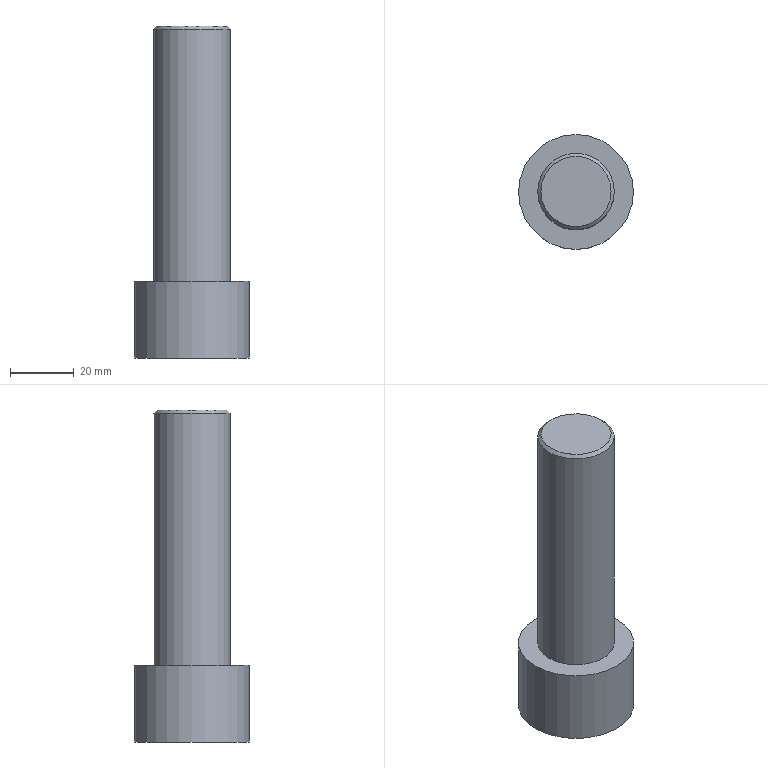Part | NX | features solid 2 | 1 solid | 16 faces | box 36 x 36 x 104 mm | volume 57183 mm3 | plane 11 | cylinder 4 | cone 1 | commonest cylinder face diameters 21.98 x1 22 x1 24 x1 36 x1
STEP:
#1=CARTESIAN_POINT('',(1313.5,-386.31,231.));
#2=VERTEX_POINT('',#1);
#3=CARTESIAN_POINT('',(1325.5,-386.31,231.));
#4=DIRECTION('',(0.,0.,-1.));
#5=DIRECTION('',(-1.,0.,0.));
#6=AXIS2_PLACEMENT_3D('',#3,#4,#5);
#7=CIRCLE('',#6,12.);
#8=EDGE_CURVE('',#2,#2,#7,.T.);
#9=ORIENTED_EDGE('',*,*,#8,.T.);
#10=EDGE_LOOP('',(#9));
#11=FACE_BOUND('',#10,.T.);
#12=CARTESIAN_POINT('',(1313.5,-386.31,152.));
#13=VERTEX_POINT('',#12);
#14=CARTESIAN_POINT('',(1325.5,-386.31,152.));
#15=DIRECTION('',(0.,0.,-1.));
#16=DIRECTION('',(-1.,0.,0.));
#17=AXIS2_PLACEMENT_3D('',#14,#15,#16);
#18=CIRCLE('',#17,12.);
#19=EDGE_CURVE('',#13,#13,#18,.F.);
#20=ORIENTED_EDGE('',*,*,#19,.T.);
#21=EDGE_LOOP('',(#20));
#22=FACE_BOUND('',#21,.T.);
#23=CARTESIAN_POINT('',(1325.5,-386.31,207.));
#24=DIRECTION('',(0.,0.,1.));
#25=DIRECTION('',(-1.,0.,0.));
#26=AXIS2_PLACEMENT_3D('',#23,#24,#25);
#27=CYLINDRICAL_SURFACE('',#26,12.);
#28=ADVANCED_FACE('',(#11,#22),#27,.T.);
#29=ORIENTED_EDGE('',*,*,#19,.F.);
#30=EDGE_LOOP('',(#29));
#31=FACE_BOUND('',#30,.T.);
#32=CARTESIAN_POINT('',(1307.5,-386.31,152.));
#33=VERTEX_POINT('',#32);
#34=CARTESIAN_POINT('',(1325.5,-386.31,152.));
#35=DIRECTION('',(0.,0.,-1.));
#36=DIRECTION('',(-1.,0.,0.));
#37=AXIS2_PLACEMENT_3D('',#34,#35,#36);
#38=CIRCLE('',#37,18.);
#39=EDGE_CURVE('',#33,#33,#38,.T.);
#40=ORIENTED_EDGE('',*,*,#39,.F.);
#41=EDGE_LOOP('',(#40));
#42=FACE_BOUND('',#41,.T.);
#43=CARTESIAN_POINT('',(1325.5,-386.31,152.));
#44=DIRECTION('',(0.,0.,1.));
#45=DIRECTION('',(-1.,0.,0.));
#46=AXIS2_PLACEMENT_3D('',#43,#44,#45);
#47=PLANE('',#46);
#48=ADVANCED_FACE('',(#31,#42),#47,.T.);
#49=CARTESIAN_POINT('',(1315.108,-386.31,128.));
#50=VERTEX_POINT('',#49);
#51=CARTESIAN_POINT('',(1320.304,-377.31,128.));
#52=VERTEX_POINT('',#51);
#53=CARTESIAN_POINT('',(1320.304,-377.31,128.));
#54=DIRECTION('',(-0.5,-0.866,0.));
#55=VECTOR('',#54,1000.);
#56=LINE('',#53,#55);
#57=EDGE_CURVE('',#50,#52,#56,.F.);
#58=ORIENTED_EDGE('',*,*,#57,.F.);
#59=CARTESIAN_POINT('',(1320.304,-395.31,128.));
#60=VERTEX_POINT('',#59);
#61=CARTESIAN_POINT('',(1315.108,-386.31,128.));
#62=DIRECTION('',(0.5,-0.866,0.));
#63=VECTOR('',#62,1000.);
#64=LINE('',#61,#63);
#65=EDGE_CURVE('',#60,#50,#64,.F.);
#66=ORIENTED_EDGE('',*,*,#65,.F.);
#67=CARTESIAN_POINT('',(1330.696,-395.31,128.));
#68=VERTEX_POINT('',#67);
#69=CARTESIAN_POINT('',(1320.304,-395.31,128.));
#70=DIRECTION('',(1.,0.,0.));
#71=VECTOR('',#70,1000.);
#72=LINE('',#69,#71);
#73=EDGE_CURVE('',#68,#60,#72,.F.);
#74=ORIENTED_EDGE('',*,*,#73,.F.);
#75=CARTESIAN_POINT('',(1335.892,-386.31,128.));
#76=VERTEX_POINT('',#75);
#77=CARTESIAN_POINT('',(1330.696,-395.31,128.));
#78=DIRECTION('',(0.5,0.866,0.));
#79=VECTOR('',#78,1000.);
#80=LINE('',#77,#79);
#81=EDGE_CURVE('',#76,#68,#80,.F.);
#82=ORIENTED_EDGE('',*,*,#81,.F.);
#83=CARTESIAN_POINT('',(1330.696,-377.31,128.));
#84=VERTEX_POINT('',#83);
#85=CARTESIAN_POINT('',(1335.892,-386.31,128.));
#86=DIRECTION('',(-0.5,0.866,0.));
#87=VECTOR('',#86,1000.);
#88=LINE('',#85,#87);
#89=EDGE_CURVE('',#84,#76,#88,.F.);
#90=ORIENTED_EDGE('',*,*,#89,.F.);
#91=CARTESIAN_POINT('',(1330.696,-377.31,128.));
#92=DIRECTION('',(-1.,0.,0.));
#93=VECTOR('',#92,1000.);
#94=LINE('',#91,#93);
#95=EDGE_CURVE('',#52,#84,#94,.F.);
#96=ORIENTED_EDGE('',*,*,#95,.F.);
#97=EDGE_LOOP('',(#58,#66,#74,#82,#90,#96));
#98=FACE_BOUND('',#97,.T.);
#99=CARTESIAN_POINT('',(1343.5,-386.31,128.));
#100=VERTEX_POINT('',#99);
#101=CARTESIAN_POINT('',(1325.5,-386.31,128.));
#102=DIRECTION('',(0.,0.,1.));
#103=DIRECTION('',(1.,0.,0.));
#104=AXIS2_PLACEMENT_3D('',#101,#102,#103);
#105=CIRCLE('',#104,18.);
#106=EDGE_CURVE('',#100,#100,#105,.T.);
#107=ORIENTED_EDGE('',*,*,#106,.F.);
#108=EDGE_LOOP('',(#107));
#109=FACE_BOUND('',#108,.T.);
#110=CARTESIAN_POINT('',(1325.5,-386.31,128.));
#111=DIRECTION('',(0.,0.,-1.));
#112=DIRECTION('',(1.,0.,0.));
#113=AXIS2_PLACEMENT_3D('',#110,#111,#112);
#114=PLANE('',#113);
#115=ADVANCED_FACE('',(#98,#109),#114,.T.);
#116=ORIENTED_EDGE('',*,*,#39,.T.);
#117=EDGE_LOOP('',(#116));
#118=FACE_BOUND('',#117,.T.);
#119=ORIENTED_EDGE('',*,*,#106,.T.);
#120=EDGE_LOOP('',(#119));
#121=FACE_BOUND('',#120,.T.);
#122=CARTESIAN_POINT('',(1325.5,-386.31,126.));
#123=DIRECTION('',(0.,0.,1.));
#124=DIRECTION('',(-1.,0.,0.));
#125=AXIS2_PLACEMENT_3D('',#122,#123,#124);
#126=CYLINDRICAL_SURFACE('',#125,18.);
#127=ADVANCED_FACE('',(#118,#121),#126,.T.);
#128=CARTESIAN_POINT('',(1314.5,-386.31,232.));
#129=VERTEX_POINT('',#128);
#130=CARTESIAN_POINT('',(1325.5,-386.31,232.));
#131=DIRECTION('',(0.,0.,-1.));
#132=DIRECTION('',(-1.,0.,0.));
#133=AXIS2_PLACEMENT_3D('',#130,#131,#132);
#134=CIRCLE('',#133,11.);
#135=EDGE_CURVE('',#129,#129,#134,.F.);
#136=ORIENTED_EDGE('',*,*,#135,.F.);
#137=EDGE_LOOP('',(#136));
#138=FACE_BOUND('',#137,.T.);
#139=ORIENTED_EDGE('',*,*,#8,.F.);
#140=EDGE_LOOP('',(#139));
#141=FACE_BOUND('',#140,.T.);
#142=CARTESIAN_POINT('',(1325.5,-386.31,231.));
#143=DIRECTION('',(0.,0.,-1.));
#144=DIRECTION('',(1.,0.,0.));
#145=AXIS2_PLACEMENT_3D('',#142,#143,#144);
#146=CONICAL_SURFACE('',#145,12.,0.7854);
#147=ADVANCED_FACE('',(#138,#141),#146,.T.);
#148=CARTESIAN_POINT('',(1336.49,-386.31,184.));
#149=VERTEX_POINT('',#148);
#150=CARTESIAN_POINT('',(1325.5,-386.31,184.));
#151=DIRECTION('',(0.,0.,1.));
#152=DIRECTION('',(1.,0.,0.));
#153=AXIS2_PLACEMENT_3D('',#150,#151,#152);
#154=CIRCLE('',#153,10.99);
#155=EDGE_CURVE('',#149,#149,#154,.F.);
#156=ORIENTED_EDGE('',*,*,#155,.T.);
#157=EDGE_LOOP('',(#156));
#158=FACE_BOUND('',#157,.T.);
#159=CARTESIAN_POINT('',(1314.5,-386.31,184.));
#160=VERTEX_POINT('',#159);
#161=CARTESIAN_POINT('',(1325.5,-386.31,184.));
#162=DIRECTION('',(0.,0.,-1.));
#163=DIRECTION('',(-1.,0.,0.));
#164=AXIS2_PLACEMENT_3D('',#161,#162,#163);
#165=CIRCLE('',#164,11.);
#166=EDGE_CURVE('',#160,#160,#165,.T.);
#167=ORIENTED_EDGE('',*,*,#166,.F.);
#168=EDGE_LOOP('',(#167));
#169=FACE_BOUND('',#168,.T.);
#170=CARTESIAN_POINT('',(1325.5,-386.31,184.));
#171=DIRECTION('',(0.,0.,-1.));
#172=DIRECTION('',(1.,0.,0.));
#173=AXIS2_PLACEMENT_3D('',#170,#171,#172);
#174=PLANE('',#173);
#175=ADVANCED_FACE('',(#158,#169),#174,.F.);
#176=ORIENTED_EDGE('',*,*,#155,.F.);
#177=EDGE_LOOP('',(#176));
#178=FACE_BOUND('',#177,.T.);
#179=CARTESIAN_POINT('',(1336.49,-386.31,232.));
#180=VERTEX_POINT('',#179);
#181=CARTESIAN_POINT('',(1325.5,-386.31,232.));
#182=DIRECTION('',(0.,0.,1.));
#183=DIRECTION('',(1.,0.,0.));
#184=AXIS2_PLACEMENT_3D('',#181,#182,#183);
#185=CIRCLE('',#184,10.99);
#186=EDGE_CURVE('',#180,#180,#185,.T.);
#187=ORIENTED_EDGE('',*,*,#186,.F.);
#188=EDGE_LOOP('',(#187));
#189=FACE_BOUND('',#188,.T.);
#190=CARTESIAN_POINT('',(1325.5,-386.31,232.));
#191=DIRECTION('',(0.,0.,-1.));
#192=DIRECTION('',(1.,0.,0.));
#193=AXIS2_PLACEMENT_3D('',#190,#191,#192);
#194=CYLINDRICAL_SURFACE('',#193,10.99);
#195=ADVANCED_FACE('',(#178,#189),#194,.T.);
#196=ORIENTED_EDGE('',*,*,#166,.T.);
#197=EDGE_LOOP('',(#196));
#198=FACE_BOUND('',#197,.T.);
#199=ORIENTED_EDGE('',*,*,#135,.T.);
#200=EDGE_LOOP('',(#199));
#201=FACE_BOUND('',#200,.T.);
#202=CARTESIAN_POINT('',(1325.5,-386.31,232.));
#203=DIRECTION('',(0.,0.,-1.));
#204=DIRECTION('',(1.,0.,0.));
#205=AXIS2_PLACEMENT_3D('',#202,#203,#204);
#206=CYLINDRICAL_SURFACE('',#205,11.);
#207=ADVANCED_FACE('',(#198,#201),#206,.F.);
#208=ORIENTED_EDGE('',*,*,#186,.T.);
#209=EDGE_LOOP('',(#208));
#210=FACE_BOUND('',#209,.T.);
#211=CARTESIAN_POINT('',(1325.5,-386.31,232.));
#212=DIRECTION('',(0.,0.,1.));
#213=DIRECTION('',(-1.,0.,0.));
#214=AXIS2_PLACEMENT_3D('',#211,#212,#213);
#215=PLANE('',#214);
#216=ADVANCED_FACE('',(#210),#215,.T.);
#217=ORIENTED_EDGE('',*,*,#57,.T.);
#218=CARTESIAN_POINT('',(1320.304,-377.31,140.));
#219=VERTEX_POINT('',#218);
#220=CARTESIAN_POINT('',(1320.304,-377.31,140.));
#221=DIRECTION('',(0.,0.,-1.));
#222=VECTOR('',#221,1000.);
#223=LINE('',#220,#222);
#224=EDGE_CURVE('',#219,#52,#223,.T.);
#225=ORIENTED_EDGE('',*,*,#224,.F.);
#226=CARTESIAN_POINT('',(1315.108,-386.31,140.));
#227=VERTEX_POINT('',#226);
#228=CARTESIAN_POINT('',(1320.304,-377.31,140.));
#229=DIRECTION('',(-0.5,-0.866,0.));
#230=VECTOR('',#229,1000.);
#231=LINE('',#228,#230);
#232=EDGE_CURVE('',#219,#227,#231,.T.);
#233=ORIENTED_EDGE('',*,*,#232,.T.);
#234=CARTESIAN_POINT('',(1315.108,-386.31,140.));
#235=DIRECTION('',(0.,0.,-1.));
#236=VECTOR('',#235,1000.);
#237=LINE('',#234,#236);
#238=EDGE_CURVE('',#227,#50,#237,.T.);
#239=ORIENTED_EDGE('',*,*,#238,.T.);
#240=EDGE_LOOP('',(#217,#225,#233,#239));
#241=FACE_BOUND('',#240,.T.);
#242=CARTESIAN_POINT('',(1320.304,-377.31,140.));
#243=DIRECTION('',(-0.866,0.5,0.));
#244=DIRECTION('',(-0.5,-0.866,0.));
#245=AXIS2_PLACEMENT_3D('',#242,#243,#244);
#246=PLANE('',#245);
#247=ADVANCED_FACE('',(#241),#246,.F.);
#248=ORIENTED_EDGE('',*,*,#65,.T.);
#249=ORIENTED_EDGE('',*,*,#238,.F.);
#250=CARTESIAN_POINT('',(1320.304,-395.31,140.));
#251=VERTEX_POINT('',#250);
#252=CARTESIAN_POINT('',(1315.108,-386.31,140.));
#253=DIRECTION('',(0.5,-0.866,0.));
#254=VECTOR('',#253,1000.);
#255=LINE('',#252,#254);
#256=EDGE_CURVE('',#227,#251,#255,.T.);
#257=ORIENTED_EDGE('',*,*,#256,.T.);
#258=CARTESIAN_POINT('',(1320.304,-395.31,140.));
#259=DIRECTION('',(0.,0.,-1.));
#260=VECTOR('',#259,1000.);
#261=LINE('',#258,#260);
#262=EDGE_CURVE('',#251,#60,#261,.T.);
#263=ORIENTED_EDGE('',*,*,#262,.T.);
#264=EDGE_LOOP('',(#248,#249,#257,#263));
#265=FACE_BOUND('',#264,.T.);
#266=CARTESIAN_POINT('',(1315.108,-386.31,140.));
#267=DIRECTION('',(-0.866,-0.5,0.));
#268=DIRECTION('',(0.5,-0.866,0.));
#269=AXIS2_PLACEMENT_3D('',#266,#267,#268);
#270=PLANE('',#269);
#271=ADVANCED_FACE('',(#265),#270,.F.);
#272=ORIENTED_EDGE('',*,*,#73,.T.);
#273=ORIENTED_EDGE('',*,*,#262,.F.);
#274=CARTESIAN_POINT('',(1330.696,-395.31,140.));
#275=VERTEX_POINT('',#274);
#276=CARTESIAN_POINT('',(1320.304,-395.31,140.));
#277=DIRECTION('',(1.,0.,0.));
#278=VECTOR('',#277,1000.);
#279=LINE('',#276,#278);
#280=EDGE_CURVE('',#251,#275,#279,.T.);
#281=ORIENTED_EDGE('',*,*,#280,.T.);
#282=CARTESIAN_POINT('',(1330.696,-395.31,140.));
#283=DIRECTION('',(0.,0.,-1.));
#284=VECTOR('',#283,1000.);
#285=LINE('',#282,#284);
#286=EDGE_CURVE('',#275,#68,#285,.T.);
#287=ORIENTED_EDGE('',*,*,#286,.T.);
#288=EDGE_LOOP('',(#272,#273,#281,#287));
#289=FACE_BOUND('',#288,.T.);
#290=CARTESIAN_POINT('',(1320.304,-395.31,140.));
#291=DIRECTION('',(0.,-1.,0.));
#292=DIRECTION('',(1.,0.,0.));
#293=AXIS2_PLACEMENT_3D('',#290,#291,#292);
#294=PLANE('',#293);
#295=ADVANCED_FACE('',(#289),#294,.F.);
#296=ORIENTED_EDGE('',*,*,#81,.T.);
#297=ORIENTED_EDGE('',*,*,#286,.F.);
#298=CARTESIAN_POINT('',(1335.892,-386.31,140.));
#299=VERTEX_POINT('',#298);
#300=CARTESIAN_POINT('',(1330.696,-395.31,140.));
#301=DIRECTION('',(0.5,0.866,0.));
#302=VECTOR('',#301,1000.);
#303=LINE('',#300,#302);
#304=EDGE_CURVE('',#275,#299,#303,.T.);
#305=ORIENTED_EDGE('',*,*,#304,.T.);
#306=CARTESIAN_POINT('',(1335.892,-386.31,140.));
#307=DIRECTION('',(0.,0.,-1.));
#308=VECTOR('',#307,1000.);
#309=LINE('',#306,#308);
#310=EDGE_CURVE('',#299,#76,#309,.T.);
#311=ORIENTED_EDGE('',*,*,#310,.T.);
#312=EDGE_LOOP('',(#296,#297,#305,#311));
#313=FACE_BOUND('',#312,.T.);
#314=CARTESIAN_POINT('',(1330.696,-395.31,140.));
#315=DIRECTION('',(0.866,-0.5,0.));
#316=DIRECTION('',(0.5,0.866,0.));
#317=AXIS2_PLACEMENT_3D('',#314,#315,#316);
#318=PLANE('',#317);
#319=ADVANCED_FACE('',(#313),#318,.F.);
#320=ORIENTED_EDGE('',*,*,#89,.T.);
#321=ORIENTED_EDGE('',*,*,#310,.F.);
#322=CARTESIAN_POINT('',(1330.696,-377.31,140.));
#323=VERTEX_POINT('',#322);
#324=CARTESIAN_POINT('',(1335.892,-386.31,140.));
#325=DIRECTION('',(-0.5,0.866,0.));
#326=VECTOR('',#325,1000.);
#327=LINE('',#324,#326);
#328=EDGE_CURVE('',#299,#323,#327,.T.);
#329=ORIENTED_EDGE('',*,*,#328,.T.);
#330=CARTESIAN_POINT('',(1330.696,-377.31,140.));
#331=DIRECTION('',(0.,0.,-1.));
#332=VECTOR('',#331,1000.);
#333=LINE('',#330,#332);
#334=EDGE_CURVE('',#323,#84,#333,.T.);
#335=ORIENTED_EDGE('',*,*,#334,.T.);
#336=EDGE_LOOP('',(#320,#321,#329,#335));
#337=FACE_BOUND('',#336,.T.);
#338=CARTESIAN_POINT('',(1335.892,-386.31,140.));
#339=DIRECTION('',(0.866,0.5,0.));
#340=DIRECTION('',(-0.5,0.866,0.));
#341=AXIS2_PLACEMENT_3D('',#338,#339,#340);
#342=PLANE('',#341);
#343=ADVANCED_FACE('',(#337),#342,.F.);
#344=ORIENTED_EDGE('',*,*,#95,.T.);
#345=ORIENTED_EDGE('',*,*,#334,.F.);
#346=CARTESIAN_POINT('',(1330.696,-377.31,140.));
#347=DIRECTION('',(-1.,0.,0.));
#348=VECTOR('',#347,1000.);
#349=LINE('',#346,#348);
#350=EDGE_CURVE('',#323,#219,#349,.T.);
#351=ORIENTED_EDGE('',*,*,#350,.T.);
#352=ORIENTED_EDGE('',*,*,#224,.T.);
#353=EDGE_LOOP('',(#344,#345,#351,#352));
#354=FACE_BOUND('',#353,.T.);
#355=CARTESIAN_POINT('',(1330.696,-377.31,140.));
#356=DIRECTION('',(0.,1.,0.));
#357=DIRECTION('',(-1.,0.,0.));
#358=AXIS2_PLACEMENT_3D('',#355,#356,#357);
#359=PLANE('',#358);
#360=ADVANCED_FACE('',(#354),#359,.F.);
#361=ORIENTED_EDGE('',*,*,#232,.F.);
#362=ORIENTED_EDGE('',*,*,#350,.F.);
#363=ORIENTED_EDGE('',*,*,#328,.F.);
#364=ORIENTED_EDGE('',*,*,#304,.F.);
#365=ORIENTED_EDGE('',*,*,#280,.F.);
#366=ORIENTED_EDGE('',*,*,#256,.F.);
#367=EDGE_LOOP('',(#361,#362,#363,#364,#365,#366));
#368=FACE_BOUND('',#367,.T.);
#369=CARTESIAN_POINT('',(1309.912,-395.31,140.));
#370=DIRECTION('',(0.,0.,-1.));
#371=DIRECTION('',(1.,0.,0.));
#372=AXIS2_PLACEMENT_3D('',#369,#370,#371);
#373=PLANE('',#372);
#374=ADVANCED_FACE('',(#368),#373,.T.);
#375=CLOSED_SHELL('',(#28,#48,#115,#127,#147,#175,#195,#207,#216,#247,#271,#295,#319,#343,#360,#374));
#376=MANIFOLD_SOLID_BREP('',#375);
#377=(LENGTH_UNIT()NAMED_UNIT(*)SI_UNIT(.MILLI.,.METRE.));
#378=UNCERTAINTY_MEASURE_WITH_UNIT(LENGTH_MEASURE(0.00001),#377,'','');
#379=(NAMED_UNIT(*)PLANE_ANGLE_UNIT()SI_UNIT($,.RADIAN.));
#380=(NAMED_UNIT(*)SI_UNIT($,.STERADIAN.)SOLID_ANGLE_UNIT());
#381=(GEOMETRIC_REPRESENTATION_CONTEXT(3)GLOBAL_UNCERTAINTY_ASSIGNED_CONTEXT((#378))GLOBAL_UNIT_ASSIGNED_CONTEXT((#377,#379,#380))REPRESENTATION_CONTEXT('',''));
#382=ADVANCED_BREP_SHAPE_REPRESENTATION('',(#376),#381);